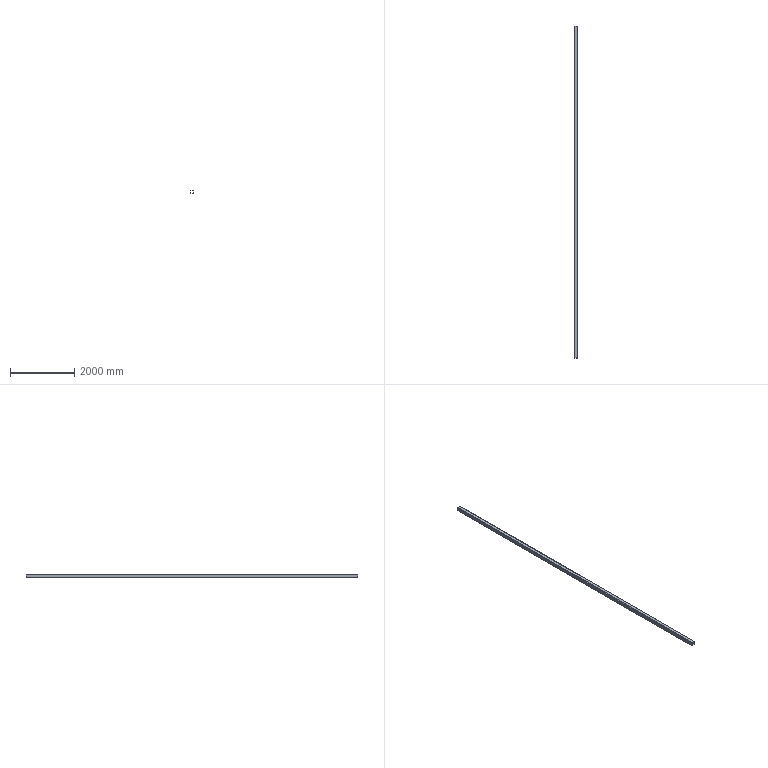Part | SolidWorks | features WeldMemberFeat 1, WeldmentFeature 1 | 1 solid | 18 faces | box 120 x 10370 x 120 mm | volume 43669629 mm3 | plane 10 | cylinder 8 | commonest cylinder face diameters 12 x4 32 x4
STEP:
#1=CARTESIAN_POINT('',(-60.,0.,44.));
#2=VERTEX_POINT('',#1);
#3=CARTESIAN_POINT('',(-44.,0.,60.));
#4=VERTEX_POINT('',#3);
#5=CARTESIAN_POINT('',(-44.,0.,44.));
#6=DIRECTION('',(0.,1.,0.));
#7=DIRECTION('',(0.,0.,1.));
#8=AXIS2_PLACEMENT_3D('',#5,#6,#7);
#9=CIRCLE('',#8,16.);
#10=EDGE_CURVE('',#2,#4,#9,.T.);
#11=ORIENTED_EDGE('',*,*,#10,.T.);
#12=CARTESIAN_POINT('',(-44.,10370.,60.));
#13=VERTEX_POINT('',#12);
#14=CARTESIAN_POINT('',(-44.,10370.,60.));
#15=DIRECTION('',(0.,-1.,0.));
#16=VECTOR('',#15,1000.);
#17=LINE('',#14,#16);
#18=EDGE_CURVE('',#13,#4,#17,.T.);
#19=ORIENTED_EDGE('',*,*,#18,.F.);
#20=CARTESIAN_POINT('',(-60.,10370.,44.));
#21=VERTEX_POINT('',#20);
#22=CARTESIAN_POINT('',(-44.,10370.,44.));
#23=DIRECTION('',(0.,1.,0.));
#24=DIRECTION('',(0.,0.,1.));
#25=AXIS2_PLACEMENT_3D('',#22,#23,#24);
#26=CIRCLE('',#25,16.);
#27=EDGE_CURVE('',#21,#13,#26,.T.);
#28=ORIENTED_EDGE('',*,*,#27,.F.);
#29=CARTESIAN_POINT('',(-60.,10370.,44.));
#30=DIRECTION('',(0.,-1.,0.));
#31=VECTOR('',#30,1000.);
#32=LINE('',#29,#31);
#33=EDGE_CURVE('',#21,#2,#32,.T.);
#34=ORIENTED_EDGE('',*,*,#33,.T.);
#35=EDGE_LOOP('',(#11,#19,#28,#34));
#36=FACE_OUTER_BOUND('',#35,.T.);
#37=CARTESIAN_POINT('',(-44.,10370.,44.));
#38=DIRECTION('',(0.,-1.,0.));
#39=DIRECTION('',(0.,0.,-1.));
#40=AXIS2_PLACEMENT_3D('',#37,#38,#39);
#41=CYLINDRICAL_SURFACE('',#40,16.);
#42=ADVANCED_FACE('',(#36),#41,.T.);
#43=CARTESIAN_POINT('',(44.,0.,60.));
#44=VERTEX_POINT('',#43);
#45=CARTESIAN_POINT('',(-44.,0.,60.));
#46=DIRECTION('',(1.,0.,0.));
#47=VECTOR('',#46,1000.);
#48=LINE('',#45,#47);
#49=EDGE_CURVE('',#4,#44,#48,.T.);
#50=ORIENTED_EDGE('',*,*,#49,.T.);
#51=CARTESIAN_POINT('',(44.,10370.,60.));
#52=VERTEX_POINT('',#51);
#53=CARTESIAN_POINT('',(44.,10370.,60.));
#54=DIRECTION('',(0.,-1.,0.));
#55=VECTOR('',#54,1000.);
#56=LINE('',#53,#55);
#57=EDGE_CURVE('',#52,#44,#56,.T.);
#58=ORIENTED_EDGE('',*,*,#57,.F.);
#59=CARTESIAN_POINT('',(-44.,10370.,60.));
#60=DIRECTION('',(1.,0.,0.));
#61=VECTOR('',#60,1000.);
#62=LINE('',#59,#61);
#63=EDGE_CURVE('',#13,#52,#62,.T.);
#64=ORIENTED_EDGE('',*,*,#63,.F.);
#65=ORIENTED_EDGE('',*,*,#18,.T.);
#66=EDGE_LOOP('',(#50,#58,#64,#65));
#67=FACE_OUTER_BOUND('',#66,.T.);
#68=CARTESIAN_POINT('',(-44.,10370.,60.));
#69=DIRECTION('',(0.,0.,-1.));
#70=DIRECTION('',(-1.,0.,0.));
#71=AXIS2_PLACEMENT_3D('',#68,#69,#70);
#72=PLANE('',#71);
#73=ADVANCED_FACE('',(#67),#72,.F.);
#74=CARTESIAN_POINT('',(60.,0.,44.));
#75=VERTEX_POINT('',#74);
#76=CARTESIAN_POINT('',(44.,0.,44.));
#77=DIRECTION('',(0.,1.,0.));
#78=DIRECTION('',(0.,0.,1.));
#79=AXIS2_PLACEMENT_3D('',#76,#77,#78);
#80=CIRCLE('',#79,16.);
#81=EDGE_CURVE('',#44,#75,#80,.T.);
#82=ORIENTED_EDGE('',*,*,#81,.T.);
#83=CARTESIAN_POINT('',(60.,10370.,44.));
#84=VERTEX_POINT('',#83);
#85=CARTESIAN_POINT('',(60.,10370.,44.));
#86=DIRECTION('',(0.,-1.,0.));
#87=VECTOR('',#86,1000.);
#88=LINE('',#85,#87);
#89=EDGE_CURVE('',#84,#75,#88,.T.);
#90=ORIENTED_EDGE('',*,*,#89,.F.);
#91=CARTESIAN_POINT('',(44.,10370.,44.));
#92=DIRECTION('',(0.,1.,0.));
#93=DIRECTION('',(0.,0.,1.));
#94=AXIS2_PLACEMENT_3D('',#91,#92,#93);
#95=CIRCLE('',#94,16.);
#96=EDGE_CURVE('',#52,#84,#95,.T.);
#97=ORIENTED_EDGE('',*,*,#96,.F.);
#98=ORIENTED_EDGE('',*,*,#57,.T.);
#99=EDGE_LOOP('',(#82,#90,#97,#98));
#100=FACE_OUTER_BOUND('',#99,.T.);
#101=CARTESIAN_POINT('',(44.,10370.,44.));
#102=DIRECTION('',(0.,-1.,0.));
#103=DIRECTION('',(0.,0.,-1.));
#104=AXIS2_PLACEMENT_3D('',#101,#102,#103);
#105=CYLINDRICAL_SURFACE('',#104,16.);
#106=ADVANCED_FACE('',(#100),#105,.T.);
#107=CARTESIAN_POINT('',(60.,0.,-44.));
#108=VERTEX_POINT('',#107);
#109=CARTESIAN_POINT('',(60.,0.,-44.));
#110=DIRECTION('',(0.,0.,-1.));
#111=VECTOR('',#110,1000.);
#112=LINE('',#109,#111);
#113=EDGE_CURVE('',#75,#108,#112,.T.);
#114=ORIENTED_EDGE('',*,*,#113,.T.);
#115=CARTESIAN_POINT('',(60.,10370.,-44.));
#116=VERTEX_POINT('',#115);
#117=CARTESIAN_POINT('',(60.,10370.,-44.));
#118=DIRECTION('',(0.,-1.,0.));
#119=VECTOR('',#118,1000.);
#120=LINE('',#117,#119);
#121=EDGE_CURVE('',#116,#108,#120,.T.);
#122=ORIENTED_EDGE('',*,*,#121,.F.);
#123=CARTESIAN_POINT('',(60.,10370.,-44.));
#124=DIRECTION('',(0.,0.,-1.));
#125=VECTOR('',#124,1000.);
#126=LINE('',#123,#125);
#127=EDGE_CURVE('',#84,#116,#126,.T.);
#128=ORIENTED_EDGE('',*,*,#127,.F.);
#129=ORIENTED_EDGE('',*,*,#89,.T.);
#130=EDGE_LOOP('',(#114,#122,#128,#129));
#131=FACE_OUTER_BOUND('',#130,.T.);
#132=CARTESIAN_POINT('',(60.,10370.,-44.));
#133=DIRECTION('',(-1.,0.,0.));
#134=DIRECTION('',(0.,0.,1.));
#135=AXIS2_PLACEMENT_3D('',#132,#133,#134);
#136=PLANE('',#135);
#137=ADVANCED_FACE('',(#131),#136,.F.);
#138=CARTESIAN_POINT('',(44.,0.,-60.));
#139=VERTEX_POINT('',#138);
#140=CARTESIAN_POINT('',(44.,0.,-44.));
#141=DIRECTION('',(0.,1.,0.));
#142=DIRECTION('',(0.,0.,1.));
#143=AXIS2_PLACEMENT_3D('',#140,#141,#142);
#144=CIRCLE('',#143,16.);
#145=EDGE_CURVE('',#108,#139,#144,.T.);
#146=ORIENTED_EDGE('',*,*,#145,.T.);
#147=CARTESIAN_POINT('',(44.,10370.,-60.));
#148=VERTEX_POINT('',#147);
#149=CARTESIAN_POINT('',(44.,10370.,-60.));
#150=DIRECTION('',(0.,-1.,0.));
#151=VECTOR('',#150,1000.);
#152=LINE('',#149,#151);
#153=EDGE_CURVE('',#148,#139,#152,.T.);
#154=ORIENTED_EDGE('',*,*,#153,.F.);
#155=CARTESIAN_POINT('',(44.,10370.,-44.));
#156=DIRECTION('',(0.,1.,0.));
#157=DIRECTION('',(0.,0.,1.));
#158=AXIS2_PLACEMENT_3D('',#155,#156,#157);
#159=CIRCLE('',#158,16.);
#160=EDGE_CURVE('',#116,#148,#159,.T.);
#161=ORIENTED_EDGE('',*,*,#160,.F.);
#162=ORIENTED_EDGE('',*,*,#121,.T.);
#163=EDGE_LOOP('',(#146,#154,#161,#162));
#164=FACE_OUTER_BOUND('',#163,.T.);
#165=CARTESIAN_POINT('',(44.,10370.,-44.));
#166=DIRECTION('',(0.,-1.,0.));
#167=DIRECTION('',(0.,0.,-1.));
#168=AXIS2_PLACEMENT_3D('',#165,#166,#167);
#169=CYLINDRICAL_SURFACE('',#168,16.);
#170=ADVANCED_FACE('',(#164),#169,.T.);
#171=CARTESIAN_POINT('',(-44.,0.,-60.));
#172=VERTEX_POINT('',#171);
#173=CARTESIAN_POINT('',(44.,0.,-60.));
#174=DIRECTION('',(-1.,0.,0.));
#175=VECTOR('',#174,1000.);
#176=LINE('',#173,#175);
#177=EDGE_CURVE('',#139,#172,#176,.T.);
#178=ORIENTED_EDGE('',*,*,#177,.T.);
#179=CARTESIAN_POINT('',(-44.,10370.,-60.));
#180=VERTEX_POINT('',#179);
#181=CARTESIAN_POINT('',(-44.,10370.,-60.));
#182=DIRECTION('',(0.,-1.,0.));
#183=VECTOR('',#182,1000.);
#184=LINE('',#181,#183);
#185=EDGE_CURVE('',#180,#172,#184,.T.);
#186=ORIENTED_EDGE('',*,*,#185,.F.);
#187=CARTESIAN_POINT('',(44.,10370.,-60.));
#188=DIRECTION('',(-1.,0.,0.));
#189=VECTOR('',#188,1000.);
#190=LINE('',#187,#189);
#191=EDGE_CURVE('',#148,#180,#190,.T.);
#192=ORIENTED_EDGE('',*,*,#191,.F.);
#193=ORIENTED_EDGE('',*,*,#153,.T.);
#194=EDGE_LOOP('',(#178,#186,#192,#193));
#195=FACE_OUTER_BOUND('',#194,.T.);
#196=CARTESIAN_POINT('',(44.,10370.,-60.));
#197=DIRECTION('',(0.,0.,1.));
#198=DIRECTION('',(1.,0.,0.));
#199=AXIS2_PLACEMENT_3D('',#196,#197,#198);
#200=PLANE('',#199);
#201=ADVANCED_FACE('',(#195),#200,.F.);
#202=CARTESIAN_POINT('',(-60.,0.,-44.));
#203=VERTEX_POINT('',#202);
#204=CARTESIAN_POINT('',(-44.,0.,-44.));
#205=DIRECTION('',(0.,1.,0.));
#206=DIRECTION('',(0.,0.,1.));
#207=AXIS2_PLACEMENT_3D('',#204,#205,#206);
#208=CIRCLE('',#207,16.);
#209=EDGE_CURVE('',#172,#203,#208,.T.);
#210=ORIENTED_EDGE('',*,*,#209,.T.);
#211=CARTESIAN_POINT('',(-60.,10370.,-44.));
#212=VERTEX_POINT('',#211);
#213=CARTESIAN_POINT('',(-60.,10370.,-44.));
#214=DIRECTION('',(0.,-1.,0.));
#215=VECTOR('',#214,1000.);
#216=LINE('',#213,#215);
#217=EDGE_CURVE('',#212,#203,#216,.T.);
#218=ORIENTED_EDGE('',*,*,#217,.F.);
#219=CARTESIAN_POINT('',(-44.,10370.,-44.));
#220=DIRECTION('',(0.,1.,0.));
#221=DIRECTION('',(0.,0.,1.));
#222=AXIS2_PLACEMENT_3D('',#219,#220,#221);
#223=CIRCLE('',#222,16.);
#224=EDGE_CURVE('',#180,#212,#223,.T.);
#225=ORIENTED_EDGE('',*,*,#224,.F.);
#226=ORIENTED_EDGE('',*,*,#185,.T.);
#227=EDGE_LOOP('',(#210,#218,#225,#226));
#228=FACE_OUTER_BOUND('',#227,.T.);
#229=CARTESIAN_POINT('',(-44.,10370.,-44.));
#230=DIRECTION('',(0.,-1.,0.));
#231=DIRECTION('',(0.,0.,-1.));
#232=AXIS2_PLACEMENT_3D('',#229,#230,#231);
#233=CYLINDRICAL_SURFACE('',#232,16.);
#234=ADVANCED_FACE('',(#228),#233,.T.);
#235=CARTESIAN_POINT('',(44.,0.,50.));
#236=VERTEX_POINT('',#235);
#237=CARTESIAN_POINT('',(50.,0.,44.));
#238=VERTEX_POINT('',#237);
#239=CARTESIAN_POINT('',(44.,0.,44.));
#240=DIRECTION('',(0.,1.,0.));
#241=DIRECTION('',(0.,0.,1.));
#242=AXIS2_PLACEMENT_3D('',#239,#240,#241);
#243=CIRCLE('',#242,6.);
#244=EDGE_CURVE('',#236,#238,#243,.T.);
#245=ORIENTED_EDGE('',*,*,#244,.F.);
#246=CARTESIAN_POINT('',(44.,10370.,50.));
#247=VERTEX_POINT('',#246);
#248=CARTESIAN_POINT('',(44.,10370.,50.));
#249=DIRECTION('',(0.,-1.,0.));
#250=VECTOR('',#249,1000.);
#251=LINE('',#248,#250);
#252=EDGE_CURVE('',#247,#236,#251,.T.);
#253=ORIENTED_EDGE('',*,*,#252,.F.);
#254=CARTESIAN_POINT('',(50.,10370.,44.));
#255=VERTEX_POINT('',#254);
#256=CARTESIAN_POINT('',(44.,10370.,44.));
#257=DIRECTION('',(0.,1.,0.));
#258=DIRECTION('',(0.,0.,1.));
#259=AXIS2_PLACEMENT_3D('',#256,#257,#258);
#260=CIRCLE('',#259,6.);
#261=EDGE_CURVE('',#247,#255,#260,.T.);
#262=ORIENTED_EDGE('',*,*,#261,.T.);
#263=CARTESIAN_POINT('',(50.,10370.,44.));
#264=DIRECTION('',(0.,-1.,0.));
#265=VECTOR('',#264,1000.);
#266=LINE('',#263,#265);
#267=EDGE_CURVE('',#255,#238,#266,.T.);
#268=ORIENTED_EDGE('',*,*,#267,.T.);
#269=EDGE_LOOP('',(#245,#253,#262,#268));
#270=FACE_OUTER_BOUND('',#269,.T.);
#271=CARTESIAN_POINT('',(44.,10370.,44.));
#272=DIRECTION('',(0.,-1.,0.));
#273=DIRECTION('',(0.,0.,-1.));
#274=AXIS2_PLACEMENT_3D('',#271,#272,#273);
#275=CYLINDRICAL_SURFACE('',#274,6.);
#276=ADVANCED_FACE('',(#270),#275,.F.);
#277=CARTESIAN_POINT('',(-44.,0.,50.));
#278=VERTEX_POINT('',#277);
#279=CARTESIAN_POINT('',(-44.,0.,50.));
#280=DIRECTION('',(1.,0.,0.));
#281=VECTOR('',#280,1000.);
#282=LINE('',#279,#281);
#283=EDGE_CURVE('',#278,#236,#282,.T.);
#284=ORIENTED_EDGE('',*,*,#283,.F.);
#285=CARTESIAN_POINT('',(-44.,10370.,50.));
#286=VERTEX_POINT('',#285);
#287=CARTESIAN_POINT('',(-44.,10370.,50.));
#288=DIRECTION('',(0.,-1.,0.));
#289=VECTOR('',#288,1000.);
#290=LINE('',#287,#289);
#291=EDGE_CURVE('',#286,#278,#290,.T.);
#292=ORIENTED_EDGE('',*,*,#291,.F.);
#293=CARTESIAN_POINT('',(-44.,10370.,50.));
#294=DIRECTION('',(1.,0.,0.));
#295=VECTOR('',#294,1000.);
#296=LINE('',#293,#295);
#297=EDGE_CURVE('',#286,#247,#296,.T.);
#298=ORIENTED_EDGE('',*,*,#297,.T.);
#299=ORIENTED_EDGE('',*,*,#252,.T.);
#300=EDGE_LOOP('',(#284,#292,#298,#299));
#301=FACE_OUTER_BOUND('',#300,.T.);
#302=CARTESIAN_POINT('',(-44.,10370.,50.));
#303=DIRECTION('',(0.,0.,-1.));
#304=DIRECTION('',(-1.,0.,0.));
#305=AXIS2_PLACEMENT_3D('',#302,#303,#304);
#306=PLANE('',#305);
#307=ADVANCED_FACE('',(#301),#306,.T.);
#308=CARTESIAN_POINT('',(-50.,0.,44.));
#309=VERTEX_POINT('',#308);
#310=CARTESIAN_POINT('',(-44.,0.,44.));
#311=DIRECTION('',(0.,1.,0.));
#312=DIRECTION('',(0.,0.,1.));
#313=AXIS2_PLACEMENT_3D('',#310,#311,#312);
#314=CIRCLE('',#313,6.);
#315=EDGE_CURVE('',#309,#278,#314,.T.);
#316=ORIENTED_EDGE('',*,*,#315,.F.);
#317=CARTESIAN_POINT('',(-50.,10370.,44.));
#318=VERTEX_POINT('',#317);
#319=CARTESIAN_POINT('',(-50.,10370.,44.));
#320=DIRECTION('',(0.,-1.,0.));
#321=VECTOR('',#320,1000.);
#322=LINE('',#319,#321);
#323=EDGE_CURVE('',#318,#309,#322,.T.);
#324=ORIENTED_EDGE('',*,*,#323,.F.);
#325=CARTESIAN_POINT('',(-44.,10370.,44.));
#326=DIRECTION('',(0.,1.,0.));
#327=DIRECTION('',(0.,0.,1.));
#328=AXIS2_PLACEMENT_3D('',#325,#326,#327);
#329=CIRCLE('',#328,6.);
#330=EDGE_CURVE('',#318,#286,#329,.T.);
#331=ORIENTED_EDGE('',*,*,#330,.T.);
#332=ORIENTED_EDGE('',*,*,#291,.T.);
#333=EDGE_LOOP('',(#316,#324,#331,#332));
#334=FACE_OUTER_BOUND('',#333,.T.);
#335=CARTESIAN_POINT('',(-44.,10370.,44.));
#336=DIRECTION('',(0.,-1.,0.));
#337=DIRECTION('',(0.,0.,-1.));
#338=AXIS2_PLACEMENT_3D('',#335,#336,#337);
#339=CYLINDRICAL_SURFACE('',#338,6.);
#340=ADVANCED_FACE('',(#334),#339,.F.);
#341=CARTESIAN_POINT('',(-50.,0.,-44.));
#342=VERTEX_POINT('',#341);
#343=CARTESIAN_POINT('',(-50.,0.,44.));
#344=DIRECTION('',(0.,0.,1.));
#345=VECTOR('',#344,1000.);
#346=LINE('',#343,#345);
#347=EDGE_CURVE('',#342,#309,#346,.T.);
#348=ORIENTED_EDGE('',*,*,#347,.F.);
#349=CARTESIAN_POINT('',(-50.,10370.,-44.));
#350=VERTEX_POINT('',#349);
#351=CARTESIAN_POINT('',(-50.,10370.,-44.));
#352=DIRECTION('',(0.,-1.,0.));
#353=VECTOR('',#352,1000.);
#354=LINE('',#351,#353);
#355=EDGE_CURVE('',#350,#342,#354,.T.);
#356=ORIENTED_EDGE('',*,*,#355,.F.);
#357=CARTESIAN_POINT('',(-50.,10370.,44.));
#358=DIRECTION('',(0.,0.,1.));
#359=VECTOR('',#358,1000.);
#360=LINE('',#357,#359);
#361=EDGE_CURVE('',#350,#318,#360,.T.);
#362=ORIENTED_EDGE('',*,*,#361,.T.);
#363=ORIENTED_EDGE('',*,*,#323,.T.);
#364=EDGE_LOOP('',(#348,#356,#362,#363));
#365=FACE_OUTER_BOUND('',#364,.T.);
#366=CARTESIAN_POINT('',(-50.,10370.,44.));
#367=DIRECTION('',(1.,0.,0.));
#368=DIRECTION('',(0.,0.,-1.));
#369=AXIS2_PLACEMENT_3D('',#366,#367,#368);
#370=PLANE('',#369);
#371=ADVANCED_FACE('',(#365),#370,.T.);
#372=CARTESIAN_POINT('',(-44.,0.,-50.));
#373=VERTEX_POINT('',#372);
#374=CARTESIAN_POINT('',(-44.,0.,-44.));
#375=DIRECTION('',(0.,1.,0.));
#376=DIRECTION('',(0.,0.,1.));
#377=AXIS2_PLACEMENT_3D('',#374,#375,#376);
#378=CIRCLE('',#377,6.);
#379=EDGE_CURVE('',#373,#342,#378,.T.);
#380=ORIENTED_EDGE('',*,*,#379,.F.);
#381=CARTESIAN_POINT('',(-44.,10370.,-50.));
#382=VERTEX_POINT('',#381);
#383=CARTESIAN_POINT('',(-44.,10370.,-50.));
#384=DIRECTION('',(0.,-1.,0.));
#385=VECTOR('',#384,1000.);
#386=LINE('',#383,#385);
#387=EDGE_CURVE('',#382,#373,#386,.T.);
#388=ORIENTED_EDGE('',*,*,#387,.F.);
#389=CARTESIAN_POINT('',(-44.,10370.,-44.));
#390=DIRECTION('',(0.,1.,0.));
#391=DIRECTION('',(0.,0.,1.));
#392=AXIS2_PLACEMENT_3D('',#389,#390,#391);
#393=CIRCLE('',#392,6.);
#394=EDGE_CURVE('',#382,#350,#393,.T.);
#395=ORIENTED_EDGE('',*,*,#394,.T.);
#396=ORIENTED_EDGE('',*,*,#355,.T.);
#397=EDGE_LOOP('',(#380,#388,#395,#396));
#398=FACE_OUTER_BOUND('',#397,.T.);
#399=CARTESIAN_POINT('',(-44.,10370.,-44.));
#400=DIRECTION('',(0.,-1.,0.));
#401=DIRECTION('',(0.,0.,-1.));
#402=AXIS2_PLACEMENT_3D('',#399,#400,#401);
#403=CYLINDRICAL_SURFACE('',#402,6.);
#404=ADVANCED_FACE('',(#398),#403,.F.);
#405=CARTESIAN_POINT('',(44.,0.,-50.));
#406=VERTEX_POINT('',#405);
#407=CARTESIAN_POINT('',(44.,0.,-50.));
#408=DIRECTION('',(-1.,0.,0.));
#409=VECTOR('',#408,1000.);
#410=LINE('',#407,#409);
#411=EDGE_CURVE('',#406,#373,#410,.T.);
#412=ORIENTED_EDGE('',*,*,#411,.F.);
#413=CARTESIAN_POINT('',(44.,10370.,-50.));
#414=VERTEX_POINT('',#413);
#415=CARTESIAN_POINT('',(44.,10370.,-50.));
#416=DIRECTION('',(0.,-1.,0.));
#417=VECTOR('',#416,1000.);
#418=LINE('',#415,#417);
#419=EDGE_CURVE('',#414,#406,#418,.T.);
#420=ORIENTED_EDGE('',*,*,#419,.F.);
#421=CARTESIAN_POINT('',(44.,10370.,-50.));
#422=DIRECTION('',(-1.,0.,0.));
#423=VECTOR('',#422,1000.);
#424=LINE('',#421,#423);
#425=EDGE_CURVE('',#414,#382,#424,.T.);
#426=ORIENTED_EDGE('',*,*,#425,.T.);
#427=ORIENTED_EDGE('',*,*,#387,.T.);
#428=EDGE_LOOP('',(#412,#420,#426,#427));
#429=FACE_OUTER_BOUND('',#428,.T.);
#430=CARTESIAN_POINT('',(44.,10370.,-50.));
#431=DIRECTION('',(0.,0.,1.));
#432=DIRECTION('',(1.,0.,0.));
#433=AXIS2_PLACEMENT_3D('',#430,#431,#432);
#434=PLANE('',#433);
#435=ADVANCED_FACE('',(#429),#434,.T.);
#436=CARTESIAN_POINT('',(50.,0.,-44.));
#437=VERTEX_POINT('',#436);
#438=CARTESIAN_POINT('',(44.,0.,-44.));
#439=DIRECTION('',(0.,1.,0.));
#440=DIRECTION('',(0.,0.,1.));
#441=AXIS2_PLACEMENT_3D('',#438,#439,#440);
#442=CIRCLE('',#441,6.);
#443=EDGE_CURVE('',#437,#406,#442,.T.);
#444=ORIENTED_EDGE('',*,*,#443,.F.);
#445=CARTESIAN_POINT('',(50.,10370.,-44.));
#446=VERTEX_POINT('',#445);
#447=CARTESIAN_POINT('',(50.,10370.,-44.));
#448=DIRECTION('',(0.,-1.,0.));
#449=VECTOR('',#448,1000.);
#450=LINE('',#447,#449);
#451=EDGE_CURVE('',#446,#437,#450,.T.);
#452=ORIENTED_EDGE('',*,*,#451,.F.);
#453=CARTESIAN_POINT('',(44.,10370.,-44.));
#454=DIRECTION('',(0.,1.,0.));
#455=DIRECTION('',(0.,0.,1.));
#456=AXIS2_PLACEMENT_3D('',#453,#454,#455);
#457=CIRCLE('',#456,6.);
#458=EDGE_CURVE('',#446,#414,#457,.T.);
#459=ORIENTED_EDGE('',*,*,#458,.T.);
#460=ORIENTED_EDGE('',*,*,#419,.T.);
#461=EDGE_LOOP('',(#444,#452,#459,#460));
#462=FACE_OUTER_BOUND('',#461,.T.);
#463=CARTESIAN_POINT('',(44.,10370.,-44.));
#464=DIRECTION('',(0.,-1.,0.));
#465=DIRECTION('',(0.,0.,-1.));
#466=AXIS2_PLACEMENT_3D('',#463,#464,#465);
#467=CYLINDRICAL_SURFACE('',#466,6.);
#468=ADVANCED_FACE('',(#462),#467,.F.);
#469=CARTESIAN_POINT('',(50.,0.,-44.));
#470=DIRECTION('',(0.,0.,-1.));
#471=VECTOR('',#470,1000.);
#472=LINE('',#469,#471);
#473=EDGE_CURVE('',#238,#437,#472,.T.);
#474=ORIENTED_EDGE('',*,*,#473,.F.);
#475=ORIENTED_EDGE('',*,*,#267,.F.);
#476=CARTESIAN_POINT('',(50.,10370.,-44.));
#477=DIRECTION('',(0.,0.,-1.));
#478=VECTOR('',#477,1000.);
#479=LINE('',#476,#478);
#480=EDGE_CURVE('',#255,#446,#479,.T.);
#481=ORIENTED_EDGE('',*,*,#480,.T.);
#482=ORIENTED_EDGE('',*,*,#451,.T.);
#483=EDGE_LOOP('',(#474,#475,#481,#482));
#484=FACE_OUTER_BOUND('',#483,.T.);
#485=CARTESIAN_POINT('',(50.,10370.,-44.));
#486=DIRECTION('',(-1.,0.,0.));
#487=DIRECTION('',(0.,0.,1.));
#488=AXIS2_PLACEMENT_3D('',#485,#486,#487);
#489=PLANE('',#488);
#490=ADVANCED_FACE('',(#484),#489,.T.);
#491=CARTESIAN_POINT('',(-60.,0.,44.));
#492=DIRECTION('',(0.,0.,1.));
#493=VECTOR('',#492,1000.);
#494=LINE('',#491,#493);
#495=EDGE_CURVE('',#203,#2,#494,.T.);
#496=ORIENTED_EDGE('',*,*,#495,.T.);
#497=ORIENTED_EDGE('',*,*,#33,.F.);
#498=CARTESIAN_POINT('',(-60.,10370.,44.));
#499=DIRECTION('',(0.,0.,1.));
#500=VECTOR('',#499,1000.);
#501=LINE('',#498,#500);
#502=EDGE_CURVE('',#212,#21,#501,.T.);
#503=ORIENTED_EDGE('',*,*,#502,.F.);
#504=ORIENTED_EDGE('',*,*,#217,.T.);
#505=EDGE_LOOP('',(#496,#497,#503,#504));
#506=FACE_OUTER_BOUND('',#505,.T.);
#507=CARTESIAN_POINT('',(-60.,10370.,44.));
#508=DIRECTION('',(1.,0.,0.));
#509=DIRECTION('',(0.,0.,-1.));
#510=AXIS2_PLACEMENT_3D('',#507,#508,#509);
#511=PLANE('',#510);
#512=ADVANCED_FACE('',(#506),#511,.F.);
#513=ORIENTED_EDGE('',*,*,#261,.F.);
#514=ORIENTED_EDGE('',*,*,#297,.F.);
#515=ORIENTED_EDGE('',*,*,#330,.F.);
#516=ORIENTED_EDGE('',*,*,#361,.F.);
#517=ORIENTED_EDGE('',*,*,#394,.F.);
#518=ORIENTED_EDGE('',*,*,#425,.F.);
#519=ORIENTED_EDGE('',*,*,#458,.F.);
#520=ORIENTED_EDGE('',*,*,#480,.F.);
#521=EDGE_LOOP('',(#513,#514,#515,#516,#517,#518,#519,#520));
#522=FACE_BOUND('',#521,.T.);
#523=ORIENTED_EDGE('',*,*,#27,.T.);
#524=ORIENTED_EDGE('',*,*,#63,.T.);
#525=ORIENTED_EDGE('',*,*,#96,.T.);
#526=ORIENTED_EDGE('',*,*,#127,.T.);
#527=ORIENTED_EDGE('',*,*,#160,.T.);
#528=ORIENTED_EDGE('',*,*,#191,.T.);
#529=ORIENTED_EDGE('',*,*,#224,.T.);
#530=ORIENTED_EDGE('',*,*,#502,.T.);
#531=EDGE_LOOP('',(#523,#524,#525,#526,#527,#528,#529,#530));
#532=FACE_OUTER_BOUND('',#531,.T.);
#533=CARTESIAN_POINT('',(-44.,10370.,44.));
#534=DIRECTION('',(0.,1.,0.));
#535=DIRECTION('',(0.,0.,1.));
#536=AXIS2_PLACEMENT_3D('',#533,#534,#535);
#537=PLANE('',#536);
#538=ADVANCED_FACE('',(#522,#532),#537,.T.);
#539=ORIENTED_EDGE('',*,*,#244,.T.);
#540=ORIENTED_EDGE('',*,*,#473,.T.);
#541=ORIENTED_EDGE('',*,*,#443,.T.);
#542=ORIENTED_EDGE('',*,*,#411,.T.);
#543=ORIENTED_EDGE('',*,*,#379,.T.);
#544=ORIENTED_EDGE('',*,*,#347,.T.);
#545=ORIENTED_EDGE('',*,*,#315,.T.);
#546=ORIENTED_EDGE('',*,*,#283,.T.);
#547=EDGE_LOOP('',(#539,#540,#541,#542,#543,#544,#545,#546));
#548=FACE_BOUND('',#547,.T.);
#549=ORIENTED_EDGE('',*,*,#10,.F.);
#550=ORIENTED_EDGE('',*,*,#495,.F.);
#551=ORIENTED_EDGE('',*,*,#209,.F.);
#552=ORIENTED_EDGE('',*,*,#177,.F.);
#553=ORIENTED_EDGE('',*,*,#145,.F.);
#554=ORIENTED_EDGE('',*,*,#113,.F.);
#555=ORIENTED_EDGE('',*,*,#81,.F.);
#556=ORIENTED_EDGE('',*,*,#49,.F.);
#557=EDGE_LOOP('',(#549,#550,#551,#552,#553,#554,#555,#556));
#558=FACE_OUTER_BOUND('',#557,.T.);
#559=CARTESIAN_POINT('',(-44.,0.,44.));
#560=DIRECTION('',(0.,1.,0.));
#561=DIRECTION('',(0.,0.,1.));
#562=AXIS2_PLACEMENT_3D('',#559,#560,#561);
#563=PLANE('',#562);
#564=ADVANCED_FACE('',(#548,#558),#563,.F.);
#565=CLOSED_SHELL('',(#42,#73,#106,#137,#170,#201,#234,#276,#307,#340,#371,#404,#435,#468,#490,#512,#538,#564));
#566=MANIFOLD_SOLID_BREP('',#565);
#567=CARTESIAN_POINT('',(0.,0.,0.));
#568=DIRECTION('',(0.,0.,1.));
#569=DIRECTION('',(1.,0.,0.));
#570=AXIS2_PLACEMENT_3D('',#567,#568,#569);
#571=(LENGTH_UNIT()NAMED_UNIT(*)SI_UNIT(.MILLI.,.METRE.));
#572=UNCERTAINTY_MEASURE_WITH_UNIT(LENGTH_MEASURE(0.00001),#571,'','');
#573=(NAMED_UNIT(*)PLANE_ANGLE_UNIT()SI_UNIT($,.RADIAN.));
#574=(NAMED_UNIT(*)SI_UNIT($,.STERADIAN.)SOLID_ANGLE_UNIT());
#575=(GEOMETRIC_REPRESENTATION_CONTEXT(3)GLOBAL_UNCERTAINTY_ASSIGNED_CONTEXT((#572))GLOBAL_UNIT_ASSIGNED_CONTEXT((#571,#573,#574))REPRESENTATION_CONTEXT('',''));
#576=ADVANCED_BREP_SHAPE_REPRESENTATION('',(#566,#570),#575);